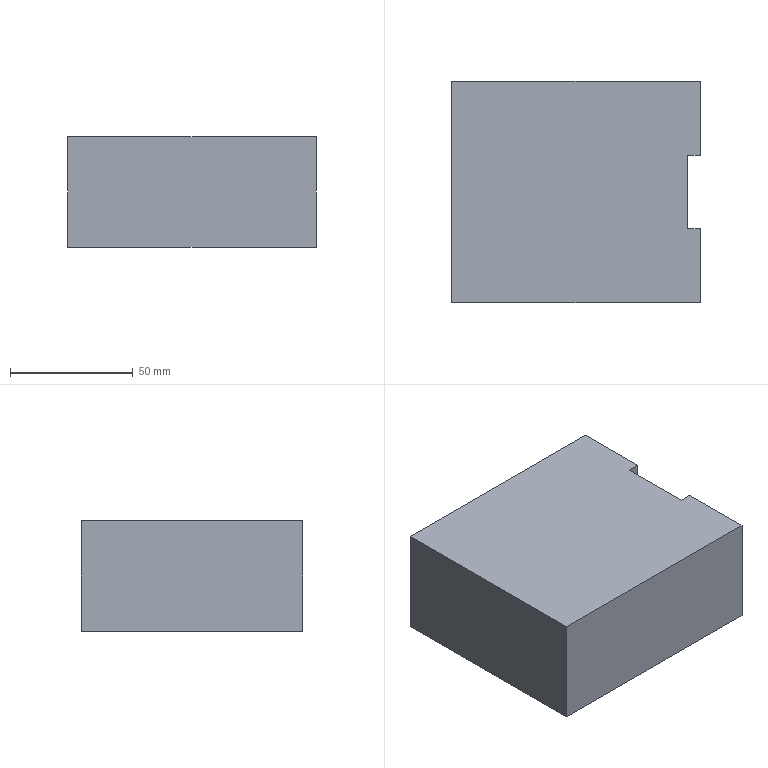Part | STEP file | DC power supply | 1 solid | 10 faces | box 101.2 x 90.2 x 45 mm | volume 404021 mm3 | plane 10
STEP:
#1=CARTESIAN_POINT('',(0.,0.,0.));
#2=DIRECTION('',(0.,0.,1.));
#3=DIRECTION('',(1.,0.,0.));
#4=AXIS2_PLACEMENT_3D('',#1,#2,#3);
#5=CARTESIAN_POINT('',(50.6,-45.1,0.));
#6=VERTEX_POINT('',#5);
#7=CARTESIAN_POINT('',(50.6,-15.,0.));
#8=VERTEX_POINT('',#7);
#9=CARTESIAN_POINT('',(50.6,45.1,0.));
#10=DIRECTION('',(0.,1.,0.));
#11=VECTOR('',#10,1.);
#12=LINE('',#9,#11);
#13=CARTESIAN_POINT('',(50.6,45.1,45.));
#14=DIRECTION('',(-1.,0.,0.));
#15=DIRECTION('',(0.,-1.,0.));
#16=AXIS2_PLACEMENT_3D('',#13,#14,#15);
#17=PLANE('',#16);
#18=CARTESIAN_POINT('',(0.,-45.));
#19=DIRECTION('',(-1.,0.));
#20=VECTOR('',#19,1.);
#21=LINE('',#18,#20);
#22=(GEOMETRIC_REPRESENTATION_CONTEXT(2)PARAMETRIC_REPRESENTATION_CONTEXT()REPRESENTATION_CONTEXT('',''));
#23=DEFINITIONAL_REPRESENTATION('',(#21),#22);
#24=PCURVE('',#17,#23);
#25=CARTESIAN_POINT('',(0.,0.,0.));
#26=DIRECTION('',(0.,0.,-1.));
#27=DIRECTION('',(-1.,0.,0.));
#28=AXIS2_PLACEMENT_3D('',#25,#26,#27);
#29=PLANE('',#28);
#30=CARTESIAN_POINT('',(-50.6,45.1));
#31=DIRECTION('',(0.,1.));
#32=VECTOR('',#31,1.);
#33=LINE('',#30,#32);
#34=(GEOMETRIC_REPRESENTATION_CONTEXT(2)PARAMETRIC_REPRESENTATION_CONTEXT()REPRESENTATION_CONTEXT('',''));
#35=DEFINITIONAL_REPRESENTATION('',(#33),#34);
#36=PCURVE('',#29,#35);
#37=SURFACE_CURVE('',#12,(#24,#36),.PCURVE_S1.);
#38=EDGE_CURVE('',#6,#8,#37,.T.);
#39=ORIENTED_EDGE('',*,*,#38,.T.);
#40=CARTESIAN_POINT('',(50.6,-15.,45.));
#41=VERTEX_POINT('',#40);
#42=CARTESIAN_POINT('',(50.6,-15.,0.));
#43=DIRECTION('',(0.,0.,1.));
#44=VECTOR('',#43,1.);
#45=LINE('',#42,#44);
#46=CARTESIAN_POINT('',(60.1,-45.));
#47=DIRECTION('',(0.,1.));
#48=VECTOR('',#47,1.);
#49=LINE('',#46,#48);
#50=(GEOMETRIC_REPRESENTATION_CONTEXT(2)PARAMETRIC_REPRESENTATION_CONTEXT()REPRESENTATION_CONTEXT('',''));
#51=DEFINITIONAL_REPRESENTATION('',(#49),#50);
#52=PCURVE('',#17,#51);
#53=CARTESIAN_POINT('',(50.6,-15.,0.));
#54=DIRECTION('',(0.,-1.,0.));
#55=DIRECTION('',(0.,0.,-1.));
#56=AXIS2_PLACEMENT_3D('',#53,#54,#55);
#57=PLANE('',#56);
#58=CARTESIAN_POINT('',(0.,0.));
#59=DIRECTION('',(-1.,0.));
#60=VECTOR('',#59,1.);
#61=LINE('',#58,#60);
#62=(GEOMETRIC_REPRESENTATION_CONTEXT(2)PARAMETRIC_REPRESENTATION_CONTEXT()REPRESENTATION_CONTEXT('',''));
#63=DEFINITIONAL_REPRESENTATION('',(#61),#62);
#64=PCURVE('',#57,#63);
#65=SURFACE_CURVE('',#45,(#52,#64),.PCURVE_S1.);
#66=EDGE_CURVE('',#8,#41,#65,.T.);
#67=ORIENTED_EDGE('',*,*,#66,.T.);
#68=CARTESIAN_POINT('',(50.6,-45.1,45.));
#69=VERTEX_POINT('',#68);
#70=CARTESIAN_POINT('',(50.6,45.1,45.));
#71=DIRECTION('',(0.,1.,0.));
#72=VECTOR('',#71,1.);
#73=LINE('',#70,#72);
#74=CARTESIAN_POINT('',(0.,0.));
#75=DIRECTION('',(-1.,0.));
#76=VECTOR('',#75,1.);
#77=LINE('',#74,#76);
#78=(GEOMETRIC_REPRESENTATION_CONTEXT(2)PARAMETRIC_REPRESENTATION_CONTEXT()REPRESENTATION_CONTEXT('',''));
#79=DEFINITIONAL_REPRESENTATION('',(#77),#78);
#80=PCURVE('',#17,#79);
#81=CARTESIAN_POINT('',(0.,0.,45.));
#82=DIRECTION('',(0.,0.,-1.));
#83=DIRECTION('',(-1.,0.,0.));
#84=AXIS2_PLACEMENT_3D('',#81,#82,#83);
#85=PLANE('',#84);
#86=CARTESIAN_POINT('',(-50.6,45.1));
#87=DIRECTION('',(0.,1.));
#88=VECTOR('',#87,1.);
#89=LINE('',#86,#88);
#90=(GEOMETRIC_REPRESENTATION_CONTEXT(2)PARAMETRIC_REPRESENTATION_CONTEXT()REPRESENTATION_CONTEXT('',''));
#91=DEFINITIONAL_REPRESENTATION('',(#89),#90);
#92=PCURVE('',#85,#91);
#93=SURFACE_CURVE('',#73,(#80,#92),.PCURVE_S1.);
#94=EDGE_CURVE('',#69,#41,#93,.T.);
#95=ORIENTED_EDGE('',*,*,#94,.F.);
#96=CARTESIAN_POINT('',(50.6,-45.1,45.));
#97=DIRECTION('',(0.,0.,-1.));
#98=VECTOR('',#97,1.);
#99=LINE('',#96,#98);
#100=CARTESIAN_POINT('',(90.2,0.));
#101=DIRECTION('',(0.,-1.));
#102=VECTOR('',#101,1.);
#103=LINE('',#100,#102);
#104=(GEOMETRIC_REPRESENTATION_CONTEXT(2)PARAMETRIC_REPRESENTATION_CONTEXT()REPRESENTATION_CONTEXT('',''));
#105=DEFINITIONAL_REPRESENTATION('',(#103),#104);
#106=PCURVE('',#17,#105);
#107=CARTESIAN_POINT('',(50.6,-45.1,45.));
#108=DIRECTION('',(0.,1.,0.));
#109=DIRECTION('',(-1.,0.,0.));
#110=AXIS2_PLACEMENT_3D('',#107,#108,#109);
#111=PLANE('',#110);
#112=CARTESIAN_POINT('',(0.,0.));
#113=DIRECTION('',(0.,-1.));
#114=VECTOR('',#113,1.);
#115=LINE('',#112,#114);
#116=(GEOMETRIC_REPRESENTATION_CONTEXT(2)PARAMETRIC_REPRESENTATION_CONTEXT()REPRESENTATION_CONTEXT('',''));
#117=DEFINITIONAL_REPRESENTATION('',(#115),#116);
#118=PCURVE('',#111,#117);
#119=SURFACE_CURVE('',#99,(#106,#118),.PCURVE_S1.);
#120=EDGE_CURVE('',#69,#6,#119,.T.);
#121=ORIENTED_EDGE('',*,*,#120,.T.);
#122=EDGE_LOOP('',(#39,#67,#95,#121));
#123=FACE_BOUND('',#122,.T.);
#124=ADVANCED_FACE('',(#123),#17,.F.);
#125=CARTESIAN_POINT('',(-50.6,45.1,0.));
#126=VERTEX_POINT('',#125);
#127=CARTESIAN_POINT('',(-50.6,-45.1,0.));
#128=VERTEX_POINT('',#127);
#129=CARTESIAN_POINT('',(-50.6,45.1,0.));
#130=DIRECTION('',(0.,-1.,0.));
#131=VECTOR('',#130,1.);
#132=LINE('',#129,#131);
#133=CARTESIAN_POINT('',(-50.6,45.1,45.));
#134=DIRECTION('',(1.,0.,0.));
#135=DIRECTION('',(0.,1.,0.));
#136=AXIS2_PLACEMENT_3D('',#133,#134,#135);
#137=PLANE('',#136);
#138=CARTESIAN_POINT('',(0.,-45.));
#139=DIRECTION('',(-1.,0.));
#140=VECTOR('',#139,1.);
#141=LINE('',#138,#140);
#142=(GEOMETRIC_REPRESENTATION_CONTEXT(2)PARAMETRIC_REPRESENTATION_CONTEXT()REPRESENTATION_CONTEXT('',''));
#143=DEFINITIONAL_REPRESENTATION('',(#141),#142);
#144=PCURVE('',#137,#143);
#145=CARTESIAN_POINT('',(50.6,45.1));
#146=DIRECTION('',(0.,-1.));
#147=VECTOR('',#146,1.);
#148=LINE('',#145,#147);
#149=(GEOMETRIC_REPRESENTATION_CONTEXT(2)PARAMETRIC_REPRESENTATION_CONTEXT()REPRESENTATION_CONTEXT('',''));
#150=DEFINITIONAL_REPRESENTATION('',(#148),#149);
#151=PCURVE('',#29,#150);
#152=SURFACE_CURVE('',#132,(#144,#151),.PCURVE_S1.);
#153=EDGE_CURVE('',#126,#128,#152,.T.);
#154=ORIENTED_EDGE('',*,*,#153,.T.);
#155=CARTESIAN_POINT('',(-50.6,-45.1,45.));
#156=VERTEX_POINT('',#155);
#157=CARTESIAN_POINT('',(-50.6,-45.1,45.));
#158=DIRECTION('',(0.,0.,-1.));
#159=VECTOR('',#158,1.);
#160=LINE('',#157,#159);
#161=CARTESIAN_POINT('',(-90.2,0.));
#162=DIRECTION('',(0.,-1.));
#163=VECTOR('',#162,1.);
#164=LINE('',#161,#163);
#165=(GEOMETRIC_REPRESENTATION_CONTEXT(2)PARAMETRIC_REPRESENTATION_CONTEXT()REPRESENTATION_CONTEXT('',''));
#166=DEFINITIONAL_REPRESENTATION('',(#164),#165);
#167=PCURVE('',#137,#166);
#168=CARTESIAN_POINT('',(101.2,0.));
#169=DIRECTION('',(0.,-1.));
#170=VECTOR('',#169,1.);
#171=LINE('',#168,#170);
#172=(GEOMETRIC_REPRESENTATION_CONTEXT(2)PARAMETRIC_REPRESENTATION_CONTEXT()REPRESENTATION_CONTEXT('',''));
#173=DEFINITIONAL_REPRESENTATION('',(#171),#172);
#174=PCURVE('',#111,#173);
#175=SURFACE_CURVE('',#160,(#167,#174),.PCURVE_S1.);
#176=EDGE_CURVE('',#156,#128,#175,.T.);
#177=ORIENTED_EDGE('',*,*,#176,.F.);
#178=CARTESIAN_POINT('',(-50.6,45.1,45.));
#179=VERTEX_POINT('',#178);
#180=CARTESIAN_POINT('',(-50.6,45.1,45.));
#181=DIRECTION('',(0.,-1.,0.));
#182=VECTOR('',#181,1.);
#183=LINE('',#180,#182);
#184=CARTESIAN_POINT('',(0.,0.));
#185=DIRECTION('',(-1.,0.));
#186=VECTOR('',#185,1.);
#187=LINE('',#184,#186);
#188=(GEOMETRIC_REPRESENTATION_CONTEXT(2)PARAMETRIC_REPRESENTATION_CONTEXT()REPRESENTATION_CONTEXT('',''));
#189=DEFINITIONAL_REPRESENTATION('',(#187),#188);
#190=PCURVE('',#137,#189);
#191=CARTESIAN_POINT('',(50.6,45.1));
#192=DIRECTION('',(0.,-1.));
#193=VECTOR('',#192,1.);
#194=LINE('',#191,#193);
#195=(GEOMETRIC_REPRESENTATION_CONTEXT(2)PARAMETRIC_REPRESENTATION_CONTEXT()REPRESENTATION_CONTEXT('',''));
#196=DEFINITIONAL_REPRESENTATION('',(#194),#195);
#197=PCURVE('',#85,#196);
#198=SURFACE_CURVE('',#183,(#190,#197),.PCURVE_S1.);
#199=EDGE_CURVE('',#179,#156,#198,.T.);
#200=ORIENTED_EDGE('',*,*,#199,.F.);
#201=CARTESIAN_POINT('',(-50.6,45.1,45.));
#202=DIRECTION('',(0.,0.,-1.));
#203=VECTOR('',#202,1.);
#204=LINE('',#201,#203);
#205=CARTESIAN_POINT('',(0.,0.));
#206=DIRECTION('',(0.,-1.));
#207=VECTOR('',#206,1.);
#208=LINE('',#205,#207);
#209=(GEOMETRIC_REPRESENTATION_CONTEXT(2)PARAMETRIC_REPRESENTATION_CONTEXT()REPRESENTATION_CONTEXT('',''));
#210=DEFINITIONAL_REPRESENTATION('',(#208),#209);
#211=PCURVE('',#137,#210);
#212=CARTESIAN_POINT('',(50.6,45.1,45.));
#213=DIRECTION('',(0.,-1.,0.));
#214=DIRECTION('',(1.,0.,0.));
#215=AXIS2_PLACEMENT_3D('',#212,#213,#214);
#216=PLANE('',#215);
#217=CARTESIAN_POINT('',(-101.2,0.));
#218=DIRECTION('',(0.,-1.));
#219=VECTOR('',#218,1.);
#220=LINE('',#217,#219);
#221=(GEOMETRIC_REPRESENTATION_CONTEXT(2)PARAMETRIC_REPRESENTATION_CONTEXT()REPRESENTATION_CONTEXT('',''));
#222=DEFINITIONAL_REPRESENTATION('',(#220),#221);
#223=PCURVE('',#216,#222);
#224=SURFACE_CURVE('',#204,(#211,#223),.PCURVE_S1.);
#225=EDGE_CURVE('',#179,#126,#224,.T.);
#226=ORIENTED_EDGE('',*,*,#225,.T.);
#227=EDGE_LOOP('',(#154,#177,#200,#226));
#228=FACE_BOUND('',#227,.T.);
#229=ADVANCED_FACE('',(#228),#137,.F.);
#230=CARTESIAN_POINT('',(50.6,-45.1,0.));
#231=DIRECTION('',(1.,0.,0.));
#232=VECTOR('',#231,1.);
#233=LINE('',#230,#232);
#234=CARTESIAN_POINT('',(0.,-45.));
#235=DIRECTION('',(-1.,0.));
#236=VECTOR('',#235,1.);
#237=LINE('',#234,#236);
#238=(GEOMETRIC_REPRESENTATION_CONTEXT(2)PARAMETRIC_REPRESENTATION_CONTEXT()REPRESENTATION_CONTEXT('',''));
#239=DEFINITIONAL_REPRESENTATION('',(#237),#238);
#240=PCURVE('',#111,#239);
#241=CARTESIAN_POINT('',(-50.6,-45.1));
#242=DIRECTION('',(-1.,0.));
#243=VECTOR('',#242,1.);
#244=LINE('',#241,#243);
#245=(GEOMETRIC_REPRESENTATION_CONTEXT(2)PARAMETRIC_REPRESENTATION_CONTEXT()REPRESENTATION_CONTEXT('',''));
#246=DEFINITIONAL_REPRESENTATION('',(#244),#245);
#247=PCURVE('',#29,#246);
#248=SURFACE_CURVE('',#233,(#240,#247),.PCURVE_S1.);
#249=EDGE_CURVE('',#128,#6,#248,.T.);
#250=ORIENTED_EDGE('',*,*,#249,.T.);
#251=ORIENTED_EDGE('',*,*,#120,.F.);
#252=CARTESIAN_POINT('',(50.6,-45.1,45.));
#253=DIRECTION('',(1.,0.,0.));
#254=VECTOR('',#253,1.);
#255=LINE('',#252,#254);
#256=CARTESIAN_POINT('',(0.,0.));
#257=DIRECTION('',(-1.,0.));
#258=VECTOR('',#257,1.);
#259=LINE('',#256,#258);
#260=(GEOMETRIC_REPRESENTATION_CONTEXT(2)PARAMETRIC_REPRESENTATION_CONTEXT()REPRESENTATION_CONTEXT('',''));
#261=DEFINITIONAL_REPRESENTATION('',(#259),#260);
#262=PCURVE('',#111,#261);
#263=CARTESIAN_POINT('',(-50.6,-45.1));
#264=DIRECTION('',(-1.,0.));
#265=VECTOR('',#264,1.);
#266=LINE('',#263,#265);
#267=(GEOMETRIC_REPRESENTATION_CONTEXT(2)PARAMETRIC_REPRESENTATION_CONTEXT()REPRESENTATION_CONTEXT('',''));
#268=DEFINITIONAL_REPRESENTATION('',(#266),#267);
#269=PCURVE('',#85,#268);
#270=SURFACE_CURVE('',#255,(#262,#269),.PCURVE_S1.);
#271=EDGE_CURVE('',#156,#69,#270,.T.);
#272=ORIENTED_EDGE('',*,*,#271,.F.);
#273=ORIENTED_EDGE('',*,*,#176,.T.);
#274=EDGE_LOOP('',(#250,#251,#272,#273));
#275=FACE_BOUND('',#274,.T.);
#276=ADVANCED_FACE('',(#275),#111,.F.);
#277=CARTESIAN_POINT('',(50.6,15.,45.));
#278=VERTEX_POINT('',#277);
#279=CARTESIAN_POINT('',(50.6,45.1,45.));
#280=VERTEX_POINT('',#279);
#281=CARTESIAN_POINT('',(50.6,45.1,45.));
#282=DIRECTION('',(0.,1.,0.));
#283=VECTOR('',#282,1.);
#284=LINE('',#281,#283);
#285=CARTESIAN_POINT('',(50.6,45.1,45.));
#286=DIRECTION('',(-1.,0.,0.));
#287=DIRECTION('',(0.,-1.,0.));
#288=AXIS2_PLACEMENT_3D('',#285,#286,#287);
#289=PLANE('',#288);
#290=CARTESIAN_POINT('',(0.,0.));
#291=DIRECTION('',(-1.,0.));
#292=VECTOR('',#291,1.);
#293=LINE('',#290,#292);
#294=(GEOMETRIC_REPRESENTATION_CONTEXT(2)PARAMETRIC_REPRESENTATION_CONTEXT()REPRESENTATION_CONTEXT('',''));
#295=DEFINITIONAL_REPRESENTATION('',(#293),#294);
#296=PCURVE('',#289,#295);
#297=CARTESIAN_POINT('',(-50.6,45.1));
#298=DIRECTION('',(0.,1.));
#299=VECTOR('',#298,1.);
#300=LINE('',#297,#299);
#301=(GEOMETRIC_REPRESENTATION_CONTEXT(2)PARAMETRIC_REPRESENTATION_CONTEXT()REPRESENTATION_CONTEXT('',''));
#302=DEFINITIONAL_REPRESENTATION('',(#300),#301);
#303=PCURVE('',#85,#302);
#304=SURFACE_CURVE('',#284,(#296,#303),.PCURVE_S1.);
#305=EDGE_CURVE('',#278,#280,#304,.T.);
#306=ORIENTED_EDGE('',*,*,#305,.F.);
#307=CARTESIAN_POINT('',(50.6,15.,0.));
#308=VERTEX_POINT('',#307);
#309=CARTESIAN_POINT('',(50.6,15.,0.));
#310=DIRECTION('',(0.,0.,1.));
#311=VECTOR('',#310,1.);
#312=LINE('',#309,#311);
#313=CARTESIAN_POINT('',(30.1,-45.));
#314=DIRECTION('',(0.,1.));
#315=VECTOR('',#314,1.);
#316=LINE('',#313,#315);
#317=(GEOMETRIC_REPRESENTATION_CONTEXT(2)PARAMETRIC_REPRESENTATION_CONTEXT()REPRESENTATION_CONTEXT('',''));
#318=DEFINITIONAL_REPRESENTATION('',(#316),#317);
#319=PCURVE('',#289,#318);
#320=CARTESIAN_POINT('',(50.6,15.,0.));
#321=DIRECTION('',(0.,1.,0.));
#322=DIRECTION('',(0.,0.,1.));
#323=AXIS2_PLACEMENT_3D('',#320,#321,#322);
#324=PLANE('',#323);
#325=CARTESIAN_POINT('',(0.,0.));
#326=DIRECTION('',(1.,0.));
#327=VECTOR('',#326,1.);
#328=LINE('',#325,#327);
#329=(GEOMETRIC_REPRESENTATION_CONTEXT(2)PARAMETRIC_REPRESENTATION_CONTEXT()REPRESENTATION_CONTEXT('',''));
#330=DEFINITIONAL_REPRESENTATION('',(#328),#329);
#331=PCURVE('',#324,#330);
#332=SURFACE_CURVE('',#312,(#319,#331),.PCURVE_S1.);
#333=EDGE_CURVE('',#308,#278,#332,.T.);
#334=ORIENTED_EDGE('',*,*,#333,.F.);
#335=CARTESIAN_POINT('',(50.6,45.1,0.));
#336=VERTEX_POINT('',#335);
#337=CARTESIAN_POINT('',(50.6,45.1,0.));
#338=DIRECTION('',(0.,1.,0.));
#339=VECTOR('',#338,1.);
#340=LINE('',#337,#339);
#341=CARTESIAN_POINT('',(0.,-45.));
#342=DIRECTION('',(-1.,0.));
#343=VECTOR('',#342,1.);
#344=LINE('',#341,#343);
#345=(GEOMETRIC_REPRESENTATION_CONTEXT(2)PARAMETRIC_REPRESENTATION_CONTEXT()REPRESENTATION_CONTEXT('',''));
#346=DEFINITIONAL_REPRESENTATION('',(#344),#345);
#347=PCURVE('',#289,#346);
#348=CARTESIAN_POINT('',(-50.6,45.1));
#349=DIRECTION('',(0.,1.));
#350=VECTOR('',#349,1.);
#351=LINE('',#348,#350);
#352=(GEOMETRIC_REPRESENTATION_CONTEXT(2)PARAMETRIC_REPRESENTATION_CONTEXT()REPRESENTATION_CONTEXT('',''));
#353=DEFINITIONAL_REPRESENTATION('',(#351),#352);
#354=PCURVE('',#29,#353);
#355=SURFACE_CURVE('',#340,(#347,#354),.PCURVE_S1.);
#356=EDGE_CURVE('',#308,#336,#355,.T.);
#357=ORIENTED_EDGE('',*,*,#356,.T.);
#358=CARTESIAN_POINT('',(50.6,45.1,45.));
#359=DIRECTION('',(0.,0.,-1.));
#360=VECTOR('',#359,1.);
#361=LINE('',#358,#360);
#362=CARTESIAN_POINT('',(0.,0.));
#363=DIRECTION('',(0.,-1.));
#364=VECTOR('',#363,1.);
#365=LINE('',#362,#364);
#366=(GEOMETRIC_REPRESENTATION_CONTEXT(2)PARAMETRIC_REPRESENTATION_CONTEXT()REPRESENTATION_CONTEXT('',''));
#367=DEFINITIONAL_REPRESENTATION('',(#365),#366);
#368=PCURVE('',#289,#367);
#369=CARTESIAN_POINT('',(0.,0.));
#370=DIRECTION('',(0.,-1.));
#371=VECTOR('',#370,1.);
#372=LINE('',#369,#371);
#373=(GEOMETRIC_REPRESENTATION_CONTEXT(2)PARAMETRIC_REPRESENTATION_CONTEXT()REPRESENTATION_CONTEXT('',''));
#374=DEFINITIONAL_REPRESENTATION('',(#372),#373);
#375=PCURVE('',#216,#374);
#376=SURFACE_CURVE('',#361,(#368,#375),.PCURVE_S1.);
#377=EDGE_CURVE('',#280,#336,#376,.T.);
#378=ORIENTED_EDGE('',*,*,#377,.F.);
#379=EDGE_LOOP('',(#306,#334,#357,#378));
#380=FACE_BOUND('',#379,.T.);
#381=ADVANCED_FACE('',(#380),#289,.F.);
#382=CARTESIAN_POINT('',(50.6,45.1,0.));
#383=DIRECTION('',(-1.,0.,0.));
#384=VECTOR('',#383,1.);
#385=LINE('',#382,#384);
#386=CARTESIAN_POINT('',(0.,-45.));
#387=DIRECTION('',(-1.,0.));
#388=VECTOR('',#387,1.);
#389=LINE('',#386,#388);
#390=(GEOMETRIC_REPRESENTATION_CONTEXT(2)PARAMETRIC_REPRESENTATION_CONTEXT()REPRESENTATION_CONTEXT('',''));
#391=DEFINITIONAL_REPRESENTATION('',(#389),#390);
#392=PCURVE('',#216,#391);
#393=CARTESIAN_POINT('',(-50.6,45.1));
#394=DIRECTION('',(1.,0.));
#395=VECTOR('',#394,1.);
#396=LINE('',#393,#395);
#397=(GEOMETRIC_REPRESENTATION_CONTEXT(2)PARAMETRIC_REPRESENTATION_CONTEXT()REPRESENTATION_CONTEXT('',''));
#398=DEFINITIONAL_REPRESENTATION('',(#396),#397);
#399=PCURVE('',#29,#398);
#400=SURFACE_CURVE('',#385,(#392,#399),.PCURVE_S1.);
#401=EDGE_CURVE('',#336,#126,#400,.T.);
#402=ORIENTED_EDGE('',*,*,#401,.T.);
#403=ORIENTED_EDGE('',*,*,#225,.F.);
#404=CARTESIAN_POINT('',(50.6,45.1,45.));
#405=DIRECTION('',(-1.,0.,0.));
#406=VECTOR('',#405,1.);
#407=LINE('',#404,#406);
#408=CARTESIAN_POINT('',(0.,0.));
#409=DIRECTION('',(-1.,0.));
#410=VECTOR('',#409,1.);
#411=LINE('',#408,#410);
#412=(GEOMETRIC_REPRESENTATION_CONTEXT(2)PARAMETRIC_REPRESENTATION_CONTEXT()REPRESENTATION_CONTEXT('',''));
#413=DEFINITIONAL_REPRESENTATION('',(#411),#412);
#414=PCURVE('',#216,#413);
#415=CARTESIAN_POINT('',(-50.6,45.1));
#416=DIRECTION('',(1.,0.));
#417=VECTOR('',#416,1.);
#418=LINE('',#415,#417);
#419=(GEOMETRIC_REPRESENTATION_CONTEXT(2)PARAMETRIC_REPRESENTATION_CONTEXT()REPRESENTATION_CONTEXT('',''));
#420=DEFINITIONAL_REPRESENTATION('',(#418),#419);
#421=PCURVE('',#85,#420);
#422=SURFACE_CURVE('',#407,(#414,#421),.PCURVE_S1.);
#423=EDGE_CURVE('',#280,#179,#422,.T.);
#424=ORIENTED_EDGE('',*,*,#423,.F.);
#425=ORIENTED_EDGE('',*,*,#377,.T.);
#426=EDGE_LOOP('',(#402,#403,#424,#425));
#427=FACE_BOUND('',#426,.T.);
#428=ADVANCED_FACE('',(#427),#216,.F.);
#429=ORIENTED_EDGE('',*,*,#94,.T.);
#430=CARTESIAN_POINT('',(45.6,-15.,45.));
#431=VERTEX_POINT('',#430);
#432=CARTESIAN_POINT('',(50.6,-15.,45.));
#433=DIRECTION('',(1.,0.,0.));
#434=VECTOR('',#433,1.);
#435=LINE('',#432,#434);
#436=CARTESIAN_POINT('',(-50.6,-15.));
#437=DIRECTION('',(-1.,0.));
#438=VECTOR('',#437,1.);
#439=LINE('',#436,#438);
#440=(GEOMETRIC_REPRESENTATION_CONTEXT(2)PARAMETRIC_REPRESENTATION_CONTEXT()REPRESENTATION_CONTEXT('',''));
#441=DEFINITIONAL_REPRESENTATION('',(#439),#440);
#442=PCURVE('',#85,#441);
#443=CARTESIAN_POINT('',(-45.,0.));
#444=DIRECTION('',(0.,1.));
#445=VECTOR('',#444,1.);
#446=LINE('',#443,#445);
#447=(GEOMETRIC_REPRESENTATION_CONTEXT(2)PARAMETRIC_REPRESENTATION_CONTEXT()REPRESENTATION_CONTEXT('',''));
#448=DEFINITIONAL_REPRESENTATION('',(#446),#447);
#449=PCURVE('',#57,#448);
#450=SURFACE_CURVE('',#435,(#442,#449),.PCURVE_S1.);
#451=EDGE_CURVE('',#431,#41,#450,.T.);
#452=ORIENTED_EDGE('',*,*,#451,.F.);
#453=CARTESIAN_POINT('',(45.6,15.,45.));
#454=VERTEX_POINT('',#453);
#455=CARTESIAN_POINT('',(45.6,15.,45.));
#456=DIRECTION('',(0.,-1.,0.));
#457=VECTOR('',#456,1.);
#458=LINE('',#455,#457);
#459=CARTESIAN_POINT('',(-45.6,15.));
#460=DIRECTION('',(0.,-1.));
#461=VECTOR('',#460,1.);
#462=LINE('',#459,#461);
#463=(GEOMETRIC_REPRESENTATION_CONTEXT(2)PARAMETRIC_REPRESENTATION_CONTEXT()REPRESENTATION_CONTEXT('',''));
#464=DEFINITIONAL_REPRESENTATION('',(#462),#463);
#465=PCURVE('',#85,#464);
#466=CARTESIAN_POINT('',(45.6,15.,0.));
#467=DIRECTION('',(-1.,0.,0.));
#468=DIRECTION('',(0.,0.,1.));
#469=AXIS2_PLACEMENT_3D('',#466,#467,#468);
#470=PLANE('',#469);
#471=CARTESIAN_POINT('',(45.,0.));
#472=DIRECTION('',(0.,-1.));
#473=VECTOR('',#472,1.);
#474=LINE('',#471,#473);
#475=(GEOMETRIC_REPRESENTATION_CONTEXT(2)PARAMETRIC_REPRESENTATION_CONTEXT()REPRESENTATION_CONTEXT('',''));
#476=DEFINITIONAL_REPRESENTATION('',(#474),#475);
#477=PCURVE('',#470,#476);
#478=SURFACE_CURVE('',#458,(#465,#477),.PCURVE_S1.);
#479=EDGE_CURVE('',#454,#431,#478,.T.);
#480=ORIENTED_EDGE('',*,*,#479,.F.);
#481=CARTESIAN_POINT('',(50.6,15.,45.));
#482=DIRECTION('',(-1.,0.,0.));
#483=VECTOR('',#482,1.);
#484=LINE('',#481,#483);
#485=CARTESIAN_POINT('',(-50.6,15.));
#486=DIRECTION('',(1.,0.));
#487=VECTOR('',#486,1.);
#488=LINE('',#485,#487);
#489=(GEOMETRIC_REPRESENTATION_CONTEXT(2)PARAMETRIC_REPRESENTATION_CONTEXT()REPRESENTATION_CONTEXT('',''));
#490=DEFINITIONAL_REPRESENTATION('',(#488),#489);
#491=PCURVE('',#85,#490);
#492=CARTESIAN_POINT('',(45.,0.));
#493=DIRECTION('',(0.,-1.));
#494=VECTOR('',#493,1.);
#495=LINE('',#492,#494);
#496=(GEOMETRIC_REPRESENTATION_CONTEXT(2)PARAMETRIC_REPRESENTATION_CONTEXT()REPRESENTATION_CONTEXT('',''));
#497=DEFINITIONAL_REPRESENTATION('',(#495),#496);
#498=PCURVE('',#324,#497);
#499=SURFACE_CURVE('',#484,(#491,#498),.PCURVE_S1.);
#500=EDGE_CURVE('',#278,#454,#499,.T.);
#501=ORIENTED_EDGE('',*,*,#500,.F.);
#502=ORIENTED_EDGE('',*,*,#305,.T.);
#503=ORIENTED_EDGE('',*,*,#423,.T.);
#504=ORIENTED_EDGE('',*,*,#199,.T.);
#505=ORIENTED_EDGE('',*,*,#271,.T.);
#506=EDGE_LOOP('',(#429,#452,#480,#501,#502,#503,#504,#505));
#507=FACE_BOUND('',#506,.T.);
#508=ADVANCED_FACE('',(#507),#85,.F.);
#509=CARTESIAN_POINT('',(45.6,-15.,0.));
#510=VERTEX_POINT('',#509);
#511=CARTESIAN_POINT('',(50.6,-15.,0.));
#512=DIRECTION('',(1.,0.,0.));
#513=VECTOR('',#512,1.);
#514=LINE('',#511,#513);
#515=CARTESIAN_POINT('',(-50.6,-15.));
#516=DIRECTION('',(-1.,0.));
#517=VECTOR('',#516,1.);
#518=LINE('',#515,#517);
#519=(GEOMETRIC_REPRESENTATION_CONTEXT(2)PARAMETRIC_REPRESENTATION_CONTEXT()REPRESENTATION_CONTEXT('',''));
#520=DEFINITIONAL_REPRESENTATION('',(#518),#519);
#521=PCURVE('',#29,#520);
#522=CARTESIAN_POINT('',(0.,0.));
#523=DIRECTION('',(0.,1.));
#524=VECTOR('',#523,1.);
#525=LINE('',#522,#524);
#526=(GEOMETRIC_REPRESENTATION_CONTEXT(2)PARAMETRIC_REPRESENTATION_CONTEXT()REPRESENTATION_CONTEXT('',''));
#527=DEFINITIONAL_REPRESENTATION('',(#525),#526);
#528=PCURVE('',#57,#527);
#529=SURFACE_CURVE('',#514,(#521,#528),.PCURVE_S1.);
#530=EDGE_CURVE('',#510,#8,#529,.T.);
#531=ORIENTED_EDGE('',*,*,#530,.T.);
#532=ORIENTED_EDGE('',*,*,#38,.F.);
#533=ORIENTED_EDGE('',*,*,#249,.F.);
#534=ORIENTED_EDGE('',*,*,#153,.F.);
#535=ORIENTED_EDGE('',*,*,#401,.F.);
#536=ORIENTED_EDGE('',*,*,#356,.F.);
#537=CARTESIAN_POINT('',(45.6,15.,0.));
#538=VERTEX_POINT('',#537);
#539=CARTESIAN_POINT('',(50.6,15.,0.));
#540=DIRECTION('',(-1.,0.,0.));
#541=VECTOR('',#540,1.);
#542=LINE('',#539,#541);
#543=CARTESIAN_POINT('',(-50.6,15.));
#544=DIRECTION('',(1.,0.));
#545=VECTOR('',#544,1.);
#546=LINE('',#543,#545);
#547=(GEOMETRIC_REPRESENTATION_CONTEXT(2)PARAMETRIC_REPRESENTATION_CONTEXT()REPRESENTATION_CONTEXT('',''));
#548=DEFINITIONAL_REPRESENTATION('',(#546),#547);
#549=PCURVE('',#29,#548);
#550=CARTESIAN_POINT('',(0.,0.));
#551=DIRECTION('',(0.,-1.));
#552=VECTOR('',#551,1.);
#553=LINE('',#550,#552);
#554=(GEOMETRIC_REPRESENTATION_CONTEXT(2)PARAMETRIC_REPRESENTATION_CONTEXT()REPRESENTATION_CONTEXT('',''));
#555=DEFINITIONAL_REPRESENTATION('',(#553),#554);
#556=PCURVE('',#324,#555);
#557=SURFACE_CURVE('',#542,(#549,#556),.PCURVE_S1.);
#558=EDGE_CURVE('',#308,#538,#557,.T.);
#559=ORIENTED_EDGE('',*,*,#558,.T.);
#560=CARTESIAN_POINT('',(45.6,15.,0.));
#561=DIRECTION('',(0.,-1.,0.));
#562=VECTOR('',#561,1.);
#563=LINE('',#560,#562);
#564=CARTESIAN_POINT('',(-45.6,15.));
#565=DIRECTION('',(0.,-1.));
#566=VECTOR('',#565,1.);
#567=LINE('',#564,#566);
#568=(GEOMETRIC_REPRESENTATION_CONTEXT(2)PARAMETRIC_REPRESENTATION_CONTEXT()REPRESENTATION_CONTEXT('',''));
#569=DEFINITIONAL_REPRESENTATION('',(#567),#568);
#570=PCURVE('',#29,#569);
#571=CARTESIAN_POINT('',(0.,0.));
#572=DIRECTION('',(0.,-1.));
#573=VECTOR('',#572,1.);
#574=LINE('',#571,#573);
#575=(GEOMETRIC_REPRESENTATION_CONTEXT(2)PARAMETRIC_REPRESENTATION_CONTEXT()REPRESENTATION_CONTEXT('',''));
#576=DEFINITIONAL_REPRESENTATION('',(#574),#575);
#577=PCURVE('',#470,#576);
#578=SURFACE_CURVE('',#563,(#570,#577),.PCURVE_S1.);
#579=EDGE_CURVE('',#538,#510,#578,.T.);
#580=ORIENTED_EDGE('',*,*,#579,.T.);
#581=EDGE_LOOP('',(#531,#532,#533,#534,#535,#536,#559,#580));
#582=FACE_BOUND('',#581,.T.);
#583=ADVANCED_FACE('',(#582),#29,.T.);
#584=ORIENTED_EDGE('',*,*,#451,.T.);
#585=ORIENTED_EDGE('',*,*,#66,.F.);
#586=ORIENTED_EDGE('',*,*,#530,.F.);
#587=CARTESIAN_POINT('',(45.6,-15.,0.));
#588=DIRECTION('',(0.,0.,1.));
#589=VECTOR('',#588,1.);
#590=LINE('',#587,#589);
#591=CARTESIAN_POINT('',(0.,-5.));
#592=DIRECTION('',(-1.,0.));
#593=VECTOR('',#592,1.);
#594=LINE('',#591,#593);
#595=(GEOMETRIC_REPRESENTATION_CONTEXT(2)PARAMETRIC_REPRESENTATION_CONTEXT()REPRESENTATION_CONTEXT('',''));
#596=DEFINITIONAL_REPRESENTATION('',(#594),#595);
#597=PCURVE('',#57,#596);
#598=CARTESIAN_POINT('',(0.,-30.));
#599=DIRECTION('',(1.,0.));
#600=VECTOR('',#599,1.);
#601=LINE('',#598,#600);
#602=(GEOMETRIC_REPRESENTATION_CONTEXT(2)PARAMETRIC_REPRESENTATION_CONTEXT()REPRESENTATION_CONTEXT('',''));
#603=DEFINITIONAL_REPRESENTATION('',(#601),#602);
#604=PCURVE('',#470,#603);
#605=SURFACE_CURVE('',#590,(#597,#604),.PCURVE_S1.);
#606=EDGE_CURVE('',#510,#431,#605,.T.);
#607=ORIENTED_EDGE('',*,*,#606,.T.);
#608=EDGE_LOOP('',(#584,#585,#586,#607));
#609=FACE_BOUND('',#608,.T.);
#610=ADVANCED_FACE('',(#609),#57,.F.);
#611=ORIENTED_EDGE('',*,*,#479,.T.);
#612=ORIENTED_EDGE('',*,*,#606,.F.);
#613=ORIENTED_EDGE('',*,*,#579,.F.);
#614=CARTESIAN_POINT('',(45.6,15.,0.));
#615=DIRECTION('',(0.,0.,1.));
#616=VECTOR('',#615,1.);
#617=LINE('',#614,#616);
#618=CARTESIAN_POINT('',(0.,0.));
#619=DIRECTION('',(1.,0.));
#620=VECTOR('',#619,1.);
#621=LINE('',#618,#620);
#622=(GEOMETRIC_REPRESENTATION_CONTEXT(2)PARAMETRIC_REPRESENTATION_CONTEXT()REPRESENTATION_CONTEXT('',''));
#623=DEFINITIONAL_REPRESENTATION('',(#621),#622);
#624=PCURVE('',#470,#623);
#625=CARTESIAN_POINT('',(0.,-5.));
#626=DIRECTION('',(1.,0.));
#627=VECTOR('',#626,1.);
#628=LINE('',#625,#627);
#629=(GEOMETRIC_REPRESENTATION_CONTEXT(2)PARAMETRIC_REPRESENTATION_CONTEXT()REPRESENTATION_CONTEXT('',''));
#630=DEFINITIONAL_REPRESENTATION('',(#628),#629);
#631=PCURVE('',#324,#630);
#632=SURFACE_CURVE('',#617,(#624,#631),.PCURVE_S1.);
#633=EDGE_CURVE('',#538,#454,#632,.T.);
#634=ORIENTED_EDGE('',*,*,#633,.T.);
#635=EDGE_LOOP('',(#611,#612,#613,#634));
#636=FACE_BOUND('',#635,.T.);
#637=ADVANCED_FACE('',(#636),#470,.F.);
#638=ORIENTED_EDGE('',*,*,#500,.T.);
#639=ORIENTED_EDGE('',*,*,#633,.F.);
#640=ORIENTED_EDGE('',*,*,#558,.F.);
#641=ORIENTED_EDGE('',*,*,#333,.T.);
#642=EDGE_LOOP('',(#638,#639,#640,#641));
#643=FACE_BOUND('',#642,.T.);
#644=ADVANCED_FACE('',(#643),#324,.F.);
#645=CLOSED_SHELL('',(#124,#229,#276,#381,#428,#508,#583,#610,#637,#644));
#646=MANIFOLD_SOLID_BREP('',#645);
#647=(LENGTH_UNIT()NAMED_UNIT(*)SI_UNIT(.MILLI.,.METRE.));
#648=UNCERTAINTY_MEASURE_WITH_UNIT(LENGTH_MEASURE(0.0000001),#647,'','');
#649=(NAMED_UNIT(*)PLANE_ANGLE_UNIT()SI_UNIT($,.RADIAN.));
#650=(NAMED_UNIT(*)SI_UNIT($,.STERADIAN.)SOLID_ANGLE_UNIT());
#651=(GEOMETRIC_REPRESENTATION_CONTEXT(3)GLOBAL_UNCERTAINTY_ASSIGNED_CONTEXT((#648))GLOBAL_UNIT_ASSIGNED_CONTEXT((#647,#649,#650))REPRESENTATION_CONTEXT('',''));
#652=ADVANCED_BREP_SHAPE_REPRESENTATION('',(#4,#646),#651);